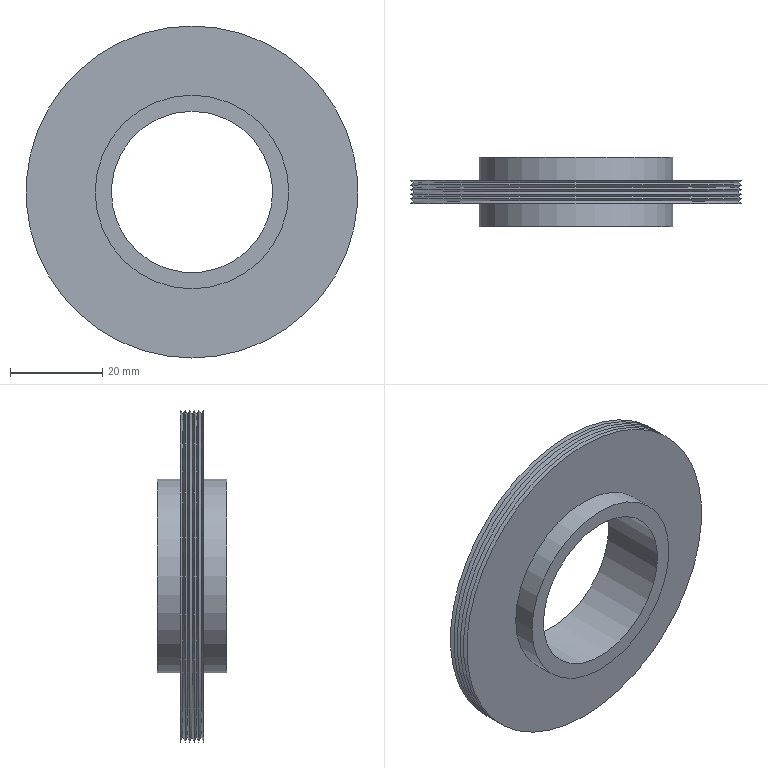Part | NX | 1 solid | 17 faces | box 72 x 15 x 72 mm | volume 19220 mm3 | cone 10 | plane 4 | cylinder 3 | commonest cylinder face diameters 42 x2 35 x1
STEP:
#1=CARTESIAN_POINT('',(0.,119.,21.));
#2=VERTEX_POINT('',#1);
#3=CARTESIAN_POINT('',(0.,119.,0.));
#4=DIRECTION('',(0.,1.,0.));
#5=DIRECTION('',(0.,0.,1.));
#6=AXIS2_PLACEMENT_3D('',#3,#4,#5);
#7=CIRCLE('',#6,21.);
#8=EDGE_CURVE('',#2,#2,#7,.T.);
#9=ORIENTED_EDGE('',*,*,#8,.F.);
#10=EDGE_LOOP('',(#9));
#11=FACE_BOUND('',#10,.T.);
#12=CARTESIAN_POINT('',(0.,114.,21.));
#13=VERTEX_POINT('',#12);
#14=CARTESIAN_POINT('',(0.,114.,0.));
#15=DIRECTION('',(0.,1.,0.));
#16=DIRECTION('',(0.,0.,1.));
#17=AXIS2_PLACEMENT_3D('',#14,#15,#16);
#18=CIRCLE('',#17,21.);
#19=EDGE_CURVE('',#13,#13,#18,.T.);
#20=ORIENTED_EDGE('',*,*,#19,.T.);
#21=EDGE_LOOP('',(#20));
#22=FACE_BOUND('',#21,.T.);
#23=CARTESIAN_POINT('',(0.,0.,0.));
#24=DIRECTION('',(0.,1.,0.));
#25=DIRECTION('',(0.,0.,-1.));
#26=AXIS2_PLACEMENT_3D('',#23,#24,#25);
#27=CYLINDRICAL_SURFACE('',#26,21.);
#28=ADVANCED_FACE('',(#11,#22),#27,.T.);
#29=CARTESIAN_POINT('',(0.,119.,36.));
#30=VERTEX_POINT('',#29);
#31=CARTESIAN_POINT('',(0.,119.,0.));
#32=DIRECTION('',(0.,1.,0.));
#33=DIRECTION('',(0.,0.,1.));
#34=AXIS2_PLACEMENT_3D('',#31,#32,#33);
#35=CIRCLE('',#34,36.);
#36=EDGE_CURVE('',#30,#30,#35,.T.);
#37=ORIENTED_EDGE('',*,*,#36,.F.);
#38=EDGE_LOOP('',(#37));
#39=FACE_BOUND('',#38,.T.);
#40=ORIENTED_EDGE('',*,*,#8,.T.);
#41=EDGE_LOOP('',(#40));
#42=FACE_BOUND('',#41,.T.);
#43=CARTESIAN_POINT('',(21.,119.,0.));
#44=DIRECTION('',(0.,1.,0.));
#45=DIRECTION('',(0.,0.,-1.));
#46=AXIS2_PLACEMENT_3D('',#43,#44,#45);
#47=PLANE('',#46);
#48=ADVANCED_FACE('',(#39,#42),#47,.F.);
#49=CARTESIAN_POINT('',(0.,119.5,35.));
#50=VERTEX_POINT('',#49);
#51=CARTESIAN_POINT('',(0.,119.5,0.));
#52=DIRECTION('',(0.,1.,0.));
#53=DIRECTION('',(0.,0.,1.));
#54=AXIS2_PLACEMENT_3D('',#51,#52,#53);
#55=CIRCLE('',#54,35.);
#56=EDGE_CURVE('',#50,#50,#55,.T.);
#57=ORIENTED_EDGE('',*,*,#56,.F.);
#58=EDGE_LOOP('',(#57));
#59=FACE_BOUND('',#58,.T.);
#60=ORIENTED_EDGE('',*,*,#36,.T.);
#61=EDGE_LOOP('',(#60));
#62=FACE_BOUND('',#61,.T.);
#63=CARTESIAN_POINT('',(0.,119.,0.));
#64=DIRECTION('',(0.,-1.,0.));
#65=DIRECTION('',(0.,0.,1.));
#66=AXIS2_PLACEMENT_3D('',#63,#64,#65);
#67=CONICAL_SURFACE('',#66,36.,63.435);
#68=ADVANCED_FACE('',(#59,#62),#67,.T.);
#69=CARTESIAN_POINT('',(0.,120.,36.));
#70=VERTEX_POINT('',#69);
#71=CARTESIAN_POINT('',(0.,120.,0.));
#72=DIRECTION('',(0.,1.,0.));
#73=DIRECTION('',(0.,0.,1.));
#74=AXIS2_PLACEMENT_3D('',#71,#72,#73);
#75=CIRCLE('',#74,36.);
#76=EDGE_CURVE('',#70,#70,#75,.T.);
#77=ORIENTED_EDGE('',*,*,#76,.F.);
#78=EDGE_LOOP('',(#77));
#79=FACE_BOUND('',#78,.T.);
#80=ORIENTED_EDGE('',*,*,#56,.T.);
#81=EDGE_LOOP('',(#80));
#82=FACE_BOUND('',#81,.T.);
#83=CARTESIAN_POINT('',(0.,119.5,0.));
#84=DIRECTION('',(0.,1.,0.));
#85=DIRECTION('',(0.,0.,-1.));
#86=AXIS2_PLACEMENT_3D('',#83,#84,#85);
#87=CONICAL_SURFACE('',#86,35.,63.435);
#88=ADVANCED_FACE('',(#79,#82),#87,.T.);
#89=CARTESIAN_POINT('',(0.,120.5,35.));
#90=VERTEX_POINT('',#89);
#91=CARTESIAN_POINT('',(0.,120.5,0.));
#92=DIRECTION('',(0.,1.,0.));
#93=DIRECTION('',(0.,0.,1.));
#94=AXIS2_PLACEMENT_3D('',#91,#92,#93);
#95=CIRCLE('',#94,35.);
#96=EDGE_CURVE('',#90,#90,#95,.T.);
#97=ORIENTED_EDGE('',*,*,#96,.F.);
#98=EDGE_LOOP('',(#97));
#99=FACE_BOUND('',#98,.T.);
#100=ORIENTED_EDGE('',*,*,#76,.T.);
#101=EDGE_LOOP('',(#100));
#102=FACE_BOUND('',#101,.T.);
#103=CARTESIAN_POINT('',(0.,120.,0.));
#104=DIRECTION('',(0.,-1.,0.));
#105=DIRECTION('',(0.,0.,1.));
#106=AXIS2_PLACEMENT_3D('',#103,#104,#105);
#107=CONICAL_SURFACE('',#106,36.,63.435);
#108=ADVANCED_FACE('',(#99,#102),#107,.T.);
#109=CARTESIAN_POINT('',(0.,121.,36.));
#110=VERTEX_POINT('',#109);
#111=CARTESIAN_POINT('',(0.,121.,0.));
#112=DIRECTION('',(0.,1.,0.));
#113=DIRECTION('',(0.,0.,1.));
#114=AXIS2_PLACEMENT_3D('',#111,#112,#113);
#115=CIRCLE('',#114,36.);
#116=EDGE_CURVE('',#110,#110,#115,.T.);
#117=ORIENTED_EDGE('',*,*,#116,.F.);
#118=EDGE_LOOP('',(#117));
#119=FACE_BOUND('',#118,.T.);
#120=ORIENTED_EDGE('',*,*,#96,.T.);
#121=EDGE_LOOP('',(#120));
#122=FACE_BOUND('',#121,.T.);
#123=CARTESIAN_POINT('',(0.,120.5,0.));
#124=DIRECTION('',(0.,1.,0.));
#125=DIRECTION('',(0.,0.,-1.));
#126=AXIS2_PLACEMENT_3D('',#123,#124,#125);
#127=CONICAL_SURFACE('',#126,35.,63.435);
#128=ADVANCED_FACE('',(#119,#122),#127,.T.);
#129=CARTESIAN_POINT('',(0.,121.5,35.));
#130=VERTEX_POINT('',#129);
#131=CARTESIAN_POINT('',(0.,121.5,0.));
#132=DIRECTION('',(0.,1.,0.));
#133=DIRECTION('',(0.,0.,1.));
#134=AXIS2_PLACEMENT_3D('',#131,#132,#133);
#135=CIRCLE('',#134,35.);
#136=EDGE_CURVE('',#130,#130,#135,.T.);
#137=ORIENTED_EDGE('',*,*,#136,.F.);
#138=EDGE_LOOP('',(#137));
#139=FACE_BOUND('',#138,.T.);
#140=ORIENTED_EDGE('',*,*,#116,.T.);
#141=EDGE_LOOP('',(#140));
#142=FACE_BOUND('',#141,.T.);
#143=CARTESIAN_POINT('',(0.,121.,0.));
#144=DIRECTION('',(0.,-1.,0.));
#145=DIRECTION('',(0.,0.,1.));
#146=AXIS2_PLACEMENT_3D('',#143,#144,#145);
#147=CONICAL_SURFACE('',#146,36.,63.435);
#148=ADVANCED_FACE('',(#139,#142),#147,.T.);
#149=CARTESIAN_POINT('',(0.,122.,36.));
#150=VERTEX_POINT('',#149);
#151=CARTESIAN_POINT('',(0.,122.,0.));
#152=DIRECTION('',(0.,1.,0.));
#153=DIRECTION('',(0.,0.,1.));
#154=AXIS2_PLACEMENT_3D('',#151,#152,#153);
#155=CIRCLE('',#154,36.);
#156=EDGE_CURVE('',#150,#150,#155,.T.);
#157=ORIENTED_EDGE('',*,*,#156,.F.);
#158=EDGE_LOOP('',(#157));
#159=FACE_BOUND('',#158,.T.);
#160=ORIENTED_EDGE('',*,*,#136,.T.);
#161=EDGE_LOOP('',(#160));
#162=FACE_BOUND('',#161,.T.);
#163=CARTESIAN_POINT('',(0.,121.5,0.));
#164=DIRECTION('',(0.,1.,0.));
#165=DIRECTION('',(0.,0.,-1.));
#166=AXIS2_PLACEMENT_3D('',#163,#164,#165);
#167=CONICAL_SURFACE('',#166,35.,63.435);
#168=ADVANCED_FACE('',(#159,#162),#167,.T.);
#169=CARTESIAN_POINT('',(0.,122.5,35.));
#170=VERTEX_POINT('',#169);
#171=CARTESIAN_POINT('',(0.,122.5,0.));
#172=DIRECTION('',(0.,1.,0.));
#173=DIRECTION('',(0.,0.,1.));
#174=AXIS2_PLACEMENT_3D('',#171,#172,#173);
#175=CIRCLE('',#174,35.);
#176=EDGE_CURVE('',#170,#170,#175,.T.);
#177=ORIENTED_EDGE('',*,*,#176,.F.);
#178=EDGE_LOOP('',(#177));
#179=FACE_BOUND('',#178,.T.);
#180=ORIENTED_EDGE('',*,*,#156,.T.);
#181=EDGE_LOOP('',(#180));
#182=FACE_BOUND('',#181,.T.);
#183=CARTESIAN_POINT('',(0.,122.,0.));
#184=DIRECTION('',(0.,-1.,0.));
#185=DIRECTION('',(0.,0.,1.));
#186=AXIS2_PLACEMENT_3D('',#183,#184,#185);
#187=CONICAL_SURFACE('',#186,36.,63.435);
#188=ADVANCED_FACE('',(#179,#182),#187,.T.);
#189=CARTESIAN_POINT('',(0.,123.,36.));
#190=VERTEX_POINT('',#189);
#191=CARTESIAN_POINT('',(0.,123.,0.));
#192=DIRECTION('',(0.,1.,0.));
#193=DIRECTION('',(0.,0.,1.));
#194=AXIS2_PLACEMENT_3D('',#191,#192,#193);
#195=CIRCLE('',#194,36.);
#196=EDGE_CURVE('',#190,#190,#195,.T.);
#197=ORIENTED_EDGE('',*,*,#196,.F.);
#198=EDGE_LOOP('',(#197));
#199=FACE_BOUND('',#198,.T.);
#200=ORIENTED_EDGE('',*,*,#176,.T.);
#201=EDGE_LOOP('',(#200));
#202=FACE_BOUND('',#201,.T.);
#203=CARTESIAN_POINT('',(0.,122.5,0.));
#204=DIRECTION('',(0.,1.,0.));
#205=DIRECTION('',(0.,0.,-1.));
#206=AXIS2_PLACEMENT_3D('',#203,#204,#205);
#207=CONICAL_SURFACE('',#206,35.,63.435);
#208=ADVANCED_FACE('',(#199,#202),#207,.T.);
#209=CARTESIAN_POINT('',(0.,123.5,35.));
#210=VERTEX_POINT('',#209);
#211=CARTESIAN_POINT('',(0.,123.5,0.));
#212=DIRECTION('',(0.,1.,0.));
#213=DIRECTION('',(0.,0.,1.));
#214=AXIS2_PLACEMENT_3D('',#211,#212,#213);
#215=CIRCLE('',#214,35.);
#216=EDGE_CURVE('',#210,#210,#215,.T.);
#217=ORIENTED_EDGE('',*,*,#216,.F.);
#218=EDGE_LOOP('',(#217));
#219=FACE_BOUND('',#218,.T.);
#220=ORIENTED_EDGE('',*,*,#196,.T.);
#221=EDGE_LOOP('',(#220));
#222=FACE_BOUND('',#221,.T.);
#223=CARTESIAN_POINT('',(0.,123.,0.));
#224=DIRECTION('',(0.,-1.,0.));
#225=DIRECTION('',(0.,0.,1.));
#226=AXIS2_PLACEMENT_3D('',#223,#224,#225);
#227=CONICAL_SURFACE('',#226,36.,63.435);
#228=ADVANCED_FACE('',(#219,#222),#227,.T.);
#229=CARTESIAN_POINT('',(0.,124.,36.));
#230=VERTEX_POINT('',#229);
#231=CARTESIAN_POINT('',(0.,124.,0.));
#232=DIRECTION('',(0.,1.,0.));
#233=DIRECTION('',(0.,0.,1.));
#234=AXIS2_PLACEMENT_3D('',#231,#232,#233);
#235=CIRCLE('',#234,36.);
#236=EDGE_CURVE('',#230,#230,#235,.T.);
#237=ORIENTED_EDGE('',*,*,#236,.F.);
#238=EDGE_LOOP('',(#237));
#239=FACE_BOUND('',#238,.T.);
#240=ORIENTED_EDGE('',*,*,#216,.T.);
#241=EDGE_LOOP('',(#240));
#242=FACE_BOUND('',#241,.T.);
#243=CARTESIAN_POINT('',(0.,123.5,0.));
#244=DIRECTION('',(0.,1.,0.));
#245=DIRECTION('',(0.,0.,-1.));
#246=AXIS2_PLACEMENT_3D('',#243,#244,#245);
#247=CONICAL_SURFACE('',#246,35.,63.435);
#248=ADVANCED_FACE('',(#239,#242),#247,.T.);
#249=CARTESIAN_POINT('',(0.,124.,21.));
#250=VERTEX_POINT('',#249);
#251=CARTESIAN_POINT('',(0.,124.,0.));
#252=DIRECTION('',(0.,1.,0.));
#253=DIRECTION('',(0.,0.,1.));
#254=AXIS2_PLACEMENT_3D('',#251,#252,#253);
#255=CIRCLE('',#254,21.);
#256=EDGE_CURVE('',#250,#250,#255,.T.);
#257=ORIENTED_EDGE('',*,*,#256,.F.);
#258=EDGE_LOOP('',(#257));
#259=FACE_BOUND('',#258,.T.);
#260=ORIENTED_EDGE('',*,*,#236,.T.);
#261=EDGE_LOOP('',(#260));
#262=FACE_BOUND('',#261,.T.);
#263=CARTESIAN_POINT('',(36.,124.,0.));
#264=DIRECTION('',(0.,-1.,0.));
#265=DIRECTION('',(0.,0.,1.));
#266=AXIS2_PLACEMENT_3D('',#263,#264,#265);
#267=PLANE('',#266);
#268=ADVANCED_FACE('',(#259,#262),#267,.F.);
#269=CARTESIAN_POINT('',(0.,129.,21.));
#270=VERTEX_POINT('',#269);
#271=CARTESIAN_POINT('',(0.,129.,0.));
#272=DIRECTION('',(0.,1.,0.));
#273=DIRECTION('',(0.,0.,1.));
#274=AXIS2_PLACEMENT_3D('',#271,#272,#273);
#275=CIRCLE('',#274,21.);
#276=EDGE_CURVE('',#270,#270,#275,.T.);
#277=ORIENTED_EDGE('',*,*,#276,.F.);
#278=EDGE_LOOP('',(#277));
#279=FACE_BOUND('',#278,.T.);
#280=ORIENTED_EDGE('',*,*,#256,.T.);
#281=EDGE_LOOP('',(#280));
#282=FACE_BOUND('',#281,.T.);
#283=CARTESIAN_POINT('',(0.,0.,0.));
#284=DIRECTION('',(0.,1.,0.));
#285=DIRECTION('',(0.,0.,-1.));
#286=AXIS2_PLACEMENT_3D('',#283,#284,#285);
#287=CYLINDRICAL_SURFACE('',#286,21.);
#288=ADVANCED_FACE('',(#279,#282),#287,.T.);
#289=CARTESIAN_POINT('',(0.,129.,17.5));
#290=VERTEX_POINT('',#289);
#291=CARTESIAN_POINT('',(0.,129.,0.));
#292=DIRECTION('',(0.,1.,0.));
#293=DIRECTION('',(0.,0.,1.));
#294=AXIS2_PLACEMENT_3D('',#291,#292,#293);
#295=CIRCLE('',#294,17.5);
#296=EDGE_CURVE('',#290,#290,#295,.T.);
#297=ORIENTED_EDGE('',*,*,#296,.F.);
#298=EDGE_LOOP('',(#297));
#299=FACE_BOUND('',#298,.T.);
#300=ORIENTED_EDGE('',*,*,#276,.T.);
#301=EDGE_LOOP('',(#300));
#302=FACE_BOUND('',#301,.T.);
#303=CARTESIAN_POINT('',(21.,129.,0.));
#304=DIRECTION('',(0.,-1.,0.));
#305=DIRECTION('',(0.,0.,1.));
#306=AXIS2_PLACEMENT_3D('',#303,#304,#305);
#307=PLANE('',#306);
#308=ADVANCED_FACE('',(#299,#302),#307,.F.);
#309=CARTESIAN_POINT('',(0.,114.,17.5));
#310=VERTEX_POINT('',#309);
#311=CARTESIAN_POINT('',(0.,114.,0.));
#312=DIRECTION('',(0.,1.,0.));
#313=DIRECTION('',(0.,0.,1.));
#314=AXIS2_PLACEMENT_3D('',#311,#312,#313);
#315=CIRCLE('',#314,17.5);
#316=EDGE_CURVE('',#310,#310,#315,.T.);
#317=ORIENTED_EDGE('',*,*,#316,.F.);
#318=EDGE_LOOP('',(#317));
#319=FACE_BOUND('',#318,.T.);
#320=ORIENTED_EDGE('',*,*,#296,.T.);
#321=EDGE_LOOP('',(#320));
#322=FACE_BOUND('',#321,.T.);
#323=CARTESIAN_POINT('',(0.,0.,0.));
#324=DIRECTION('',(0.,1.,0.));
#325=DIRECTION('',(0.,0.,-1.));
#326=AXIS2_PLACEMENT_3D('',#323,#324,#325);
#327=CYLINDRICAL_SURFACE('',#326,17.5);
#328=ADVANCED_FACE('',(#319,#322),#327,.F.);
#329=ORIENTED_EDGE('',*,*,#19,.F.);
#330=EDGE_LOOP('',(#329));
#331=FACE_BOUND('',#330,.T.);
#332=ORIENTED_EDGE('',*,*,#316,.T.);
#333=EDGE_LOOP('',(#332));
#334=FACE_BOUND('',#333,.T.);
#335=CARTESIAN_POINT('',(17.5,114.,0.));
#336=DIRECTION('',(0.,1.,0.));
#337=DIRECTION('',(0.,0.,-1.));
#338=AXIS2_PLACEMENT_3D('',#335,#336,#337);
#339=PLANE('',#338);
#340=ADVANCED_FACE('',(#331,#334),#339,.F.);
#341=CLOSED_SHELL('',(#28,#48,#68,#88,#108,#128,#148,#168,#188,#208,#228,#248,#268,#288,#308,#328,#340));
#342=MANIFOLD_SOLID_BREP('',#341);
#343=(LENGTH_UNIT()NAMED_UNIT(*)SI_UNIT(.MILLI.,.METRE.));
#344=UNCERTAINTY_MEASURE_WITH_UNIT(LENGTH_MEASURE(0.00002),#343,'','');
#345=(NAMED_UNIT(*)PLANE_ANGLE_UNIT()SI_UNIT($,.RADIAN.));
#346=PLANE_ANGLE_MEASURE_WITH_UNIT(PLANE_ANGLE_MEASURE(0.01745),#345);
#347=DIMENSIONAL_EXPONENTS(0.,0.,0.,0.,0.,0.,0.);
#348=(CONVERSION_BASED_UNIT('DEGREE',#346)NAMED_UNIT(#347)PLANE_ANGLE_UNIT());
#349=(NAMED_UNIT(*)SI_UNIT($,.STERADIAN.)SOLID_ANGLE_UNIT());
#350=(GEOMETRIC_REPRESENTATION_CONTEXT(3)GLOBAL_UNCERTAINTY_ASSIGNED_CONTEXT((#344))GLOBAL_UNIT_ASSIGNED_CONTEXT((#343,#348,#349))REPRESENTATION_CONTEXT('',''));
#351=ADVANCED_BREP_SHAPE_REPRESENTATION('',(#342),#350);